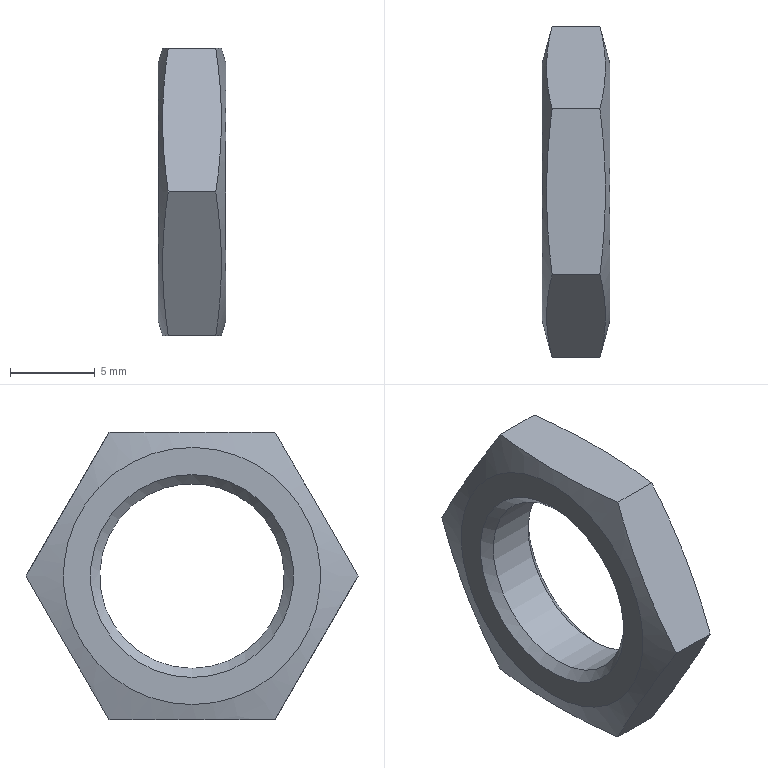Part | NX | features BREP 1 | 1 solid | 13 faces | box 4 x 19.63 x 17 mm | volume 585.312 mm3 | plane 8 | cone 4 | cylinder 1 | commonest cylinder face diameters 10.917 x1
STEP:
#1=CARTESIAN_POINT('',(4.,0.,7.6));
#2=VERTEX_POINT('',#1);
#3=CARTESIAN_POINT('',(4.,0.,0.));
#4=DIRECTION('',(-1.,0.,0.));
#5=DIRECTION('',(0.,0.,1.));
#6=AXIS2_PLACEMENT_3D('',#3,#4,#5);
#7=CIRCLE('',#6,7.6);
#8=EDGE_CURVE('',#2,#2,#7,.T.);
#9=ORIENTED_EDGE('',*,*,#8,.F.);
#10=EDGE_LOOP('',(#9));
#11=FACE_BOUND('',#10,.T.);
#12=CARTESIAN_POINT('',(4.,0.,-6.));
#13=VERTEX_POINT('',#12);
#14=CARTESIAN_POINT('',(4.,0.,0.));
#15=DIRECTION('',(1.,0.,0.));
#16=DIRECTION('',(0.,0.,-1.));
#17=AXIS2_PLACEMENT_3D('',#14,#15,#16);
#18=CIRCLE('',#17,6.);
#19=EDGE_CURVE('',#13,#13,#18,.T.);
#20=ORIENTED_EDGE('',*,*,#19,.F.);
#21=EDGE_LOOP('',(#20));
#22=FACE_BOUND('',#21,.T.);
#23=CARTESIAN_POINT('',(4.,7.6,0.));
#24=DIRECTION('',(-1.,0.,0.));
#25=DIRECTION('',(0.,0.,-1.));
#26=AXIS2_PLACEMENT_3D('',#23,#24,#25);
#27=PLANE('',#26);
#28=ADVANCED_FACE('',(#11,#22),#27,.F.);
#29=ORIENTED_EDGE('',*,*,#8,.T.);
#30=EDGE_LOOP('',(#29));
#31=FACE_BOUND('',#30,.T.);
#32=CARTESIAN_POINT('',(3.407,-9.815,0.000000038));
#33=VERTEX_POINT('',#32);
#34=CARTESIAN_POINT('',(3.407,-4.907,-8.5));
#35=VERTEX_POINT('',#34);
#36=CARTESIAN_POINT('',(3.407,-9.815,0.000000035));
#37=CARTESIAN_POINT('',(3.845,-8.179,-2.833));
#38=CARTESIAN_POINT('',(3.845,-6.543,-5.667));
#39=CARTESIAN_POINT('',(3.407,-4.907,-8.5));
#40=B_SPLINE_CURVE_WITH_KNOTS('',3,(#36,#37,#38,#39),.UNSPECIFIED.,.F.,.F.,(4,4),(0.,0.009815),.UNSPECIFIED.);
#41=EDGE_CURVE('',#33,#35,#40,.T.);
#42=ORIENTED_EDGE('',*,*,#41,.T.);
#43=CARTESIAN_POINT('',(3.407,4.907,-8.5));
#44=VERTEX_POINT('',#43);
#45=CARTESIAN_POINT('',(3.407,-4.907,-8.5));
#46=CARTESIAN_POINT('',(3.845,-1.636,-8.5));
#47=CARTESIAN_POINT('',(3.845,1.636,-8.5));
#48=CARTESIAN_POINT('',(3.407,4.907,-8.5));
#49=B_SPLINE_CURVE_WITH_KNOTS('',3,(#45,#46,#47,#48),.UNSPECIFIED.,.F.,.F.,(4,4),(0.,0.009815),.UNSPECIFIED.);
#50=EDGE_CURVE('',#35,#44,#49,.T.);
#51=ORIENTED_EDGE('',*,*,#50,.T.);
#52=CARTESIAN_POINT('',(3.407,9.815,-0.000000038));
#53=VERTEX_POINT('',#52);
#54=CARTESIAN_POINT('',(3.407,4.907,-8.5));
#55=CARTESIAN_POINT('',(3.845,6.543,-5.667));
#56=CARTESIAN_POINT('',(3.845,8.179,-2.833));
#57=CARTESIAN_POINT('',(3.407,9.815,-0.000000051));
#58=B_SPLINE_CURVE_WITH_KNOTS('',3,(#54,#55,#56,#57),.UNSPECIFIED.,.F.,.F.,(4,4),(0.,0.009815),.UNSPECIFIED.);
#59=EDGE_CURVE('',#44,#53,#58,.T.);
#60=ORIENTED_EDGE('',*,*,#59,.T.);
#61=CARTESIAN_POINT('',(3.407,4.907,8.5));
#62=VERTEX_POINT('',#61);
#63=CARTESIAN_POINT('',(3.407,9.815,-0.000000035));
#64=CARTESIAN_POINT('',(3.845,8.179,2.833));
#65=CARTESIAN_POINT('',(3.845,6.543,5.667));
#66=CARTESIAN_POINT('',(3.407,4.907,8.5));
#67=B_SPLINE_CURVE_WITH_KNOTS('',3,(#63,#64,#65,#66),.UNSPECIFIED.,.F.,.F.,(4,4),(0.,0.009815),.UNSPECIFIED.);
#68=EDGE_CURVE('',#53,#62,#67,.T.);
#69=ORIENTED_EDGE('',*,*,#68,.T.);
#70=CARTESIAN_POINT('',(3.407,-4.907,8.5));
#71=VERTEX_POINT('',#70);
#72=CARTESIAN_POINT('',(3.407,4.907,8.5));
#73=CARTESIAN_POINT('',(3.845,1.636,8.5));
#74=CARTESIAN_POINT('',(3.845,-1.636,8.5));
#75=CARTESIAN_POINT('',(3.407,-4.907,8.5));
#76=B_SPLINE_CURVE_WITH_KNOTS('',3,(#72,#73,#74,#75),.UNSPECIFIED.,.F.,.F.,(4,4),(0.,0.009815),.UNSPECIFIED.);
#77=EDGE_CURVE('',#62,#71,#76,.T.);
#78=ORIENTED_EDGE('',*,*,#77,.T.);
#79=CARTESIAN_POINT('',(3.407,-4.907,8.5));
#80=CARTESIAN_POINT('',(3.845,-6.543,5.667));
#81=CARTESIAN_POINT('',(3.845,-8.179,2.833));
#82=CARTESIAN_POINT('',(3.407,-9.815,0.000000051));
#83=B_SPLINE_CURVE_WITH_KNOTS('',3,(#79,#80,#81,#82),.UNSPECIFIED.,.F.,.F.,(4,4),(0.,0.009815),.UNSPECIFIED.);
#84=EDGE_CURVE('',#71,#33,#83,.T.);
#85=ORIENTED_EDGE('',*,*,#84,.T.);
#86=EDGE_LOOP('',(#42,#51,#60,#69,#78,#85));
#87=FACE_BOUND('',#86,.T.);
#88=CARTESIAN_POINT('',(3.403,0.,0.));
#89=DIRECTION('',(-1.,0.,0.));
#90=DIRECTION('',(0.,0.,-1.));
#91=AXIS2_PLACEMENT_3D('',#88,#89,#90);
#92=CONICAL_SURFACE('',#91,9.828,1.309);
#93=ADVANCED_FACE('',(#31,#87),#92,.T.);
#94=CARTESIAN_POINT('',(3.459,0.,-5.458));
#95=VERTEX_POINT('',#94);
#96=CARTESIAN_POINT('',(3.459,0.,0.));
#97=DIRECTION('',(1.,0.,0.));
#98=DIRECTION('',(0.,0.,-1.));
#99=AXIS2_PLACEMENT_3D('',#96,#97,#98);
#100=CIRCLE('',#99,5.458);
#101=EDGE_CURVE('',#95,#95,#100,.T.);
#102=ORIENTED_EDGE('',*,*,#101,.F.);
#103=EDGE_LOOP('',(#102));
#104=FACE_BOUND('',#103,.T.);
#105=ORIENTED_EDGE('',*,*,#19,.T.);
#106=EDGE_LOOP('',(#105));
#107=FACE_BOUND('',#106,.T.);
#108=CARTESIAN_POINT('',(4.,0.,0.));
#109=DIRECTION('',(1.,0.,0.));
#110=DIRECTION('',(0.,0.,1.));
#111=AXIS2_PLACEMENT_3D('',#108,#109,#110);
#112=CONICAL_SURFACE('',#111,6.,0.7854);
#113=ADVANCED_FACE('',(#104,#107),#112,.F.);
#114=CARTESIAN_POINT('',(0.5935,4.907,-8.5));
#115=VERTEX_POINT('',#114);
#116=CARTESIAN_POINT('',(4.,4.907,-8.5));
#117=DIRECTION('',(-1.,0.,0.));
#118=VECTOR('',#117,1000.);
#119=LINE('',#116,#118);
#120=EDGE_CURVE('',#44,#115,#119,.T.);
#121=ORIENTED_EDGE('',*,*,#120,.F.);
#122=ORIENTED_EDGE('',*,*,#50,.F.);
#123=CARTESIAN_POINT('',(0.5935,-4.907,-8.5));
#124=VERTEX_POINT('',#123);
#125=CARTESIAN_POINT('',(4.,-4.907,-8.5));
#126=DIRECTION('',(1.,0.,0.));
#127=VECTOR('',#126,1000.);
#128=LINE('',#125,#127);
#129=EDGE_CURVE('',#124,#35,#128,.T.);
#130=ORIENTED_EDGE('',*,*,#129,.F.);
#131=CARTESIAN_POINT('',(0.5935,4.907,-8.5));
#132=CARTESIAN_POINT('',(0.1552,1.636,-8.5));
#133=CARTESIAN_POINT('',(0.1552,-1.636,-8.5));
#134=CARTESIAN_POINT('',(0.5935,-4.907,-8.5));
#135=B_SPLINE_CURVE_WITH_KNOTS('',3,(#131,#132,#133,#134),.UNSPECIFIED.,.F.,.F.,(4,4),(0.,0.009815),.UNSPECIFIED.);
#136=EDGE_CURVE('',#115,#124,#135,.T.);
#137=ORIENTED_EDGE('',*,*,#136,.F.);
#138=EDGE_LOOP('',(#121,#122,#130,#137));
#139=FACE_BOUND('',#138,.T.);
#140=CARTESIAN_POINT('',(4.,-4.907,-8.5));
#141=DIRECTION('',(0.,0.,1.));
#142=DIRECTION('',(-1.,0.,0.));
#143=AXIS2_PLACEMENT_3D('',#140,#141,#142);
#144=PLANE('',#143);
#145=ADVANCED_FACE('',(#139),#144,.F.);
#146=ORIENTED_EDGE('',*,*,#41,.F.);
#147=CARTESIAN_POINT('',(0.5935,-9.815,0.));
#148=VERTEX_POINT('',#147);
#149=CARTESIAN_POINT('',(4.,-9.815,0.));
#150=DIRECTION('',(1.,0.,0.));
#151=VECTOR('',#150,1000.);
#152=LINE('',#149,#151);
#153=EDGE_CURVE('',#148,#33,#152,.T.);
#154=ORIENTED_EDGE('',*,*,#153,.F.);
#155=CARTESIAN_POINT('',(0.5935,-4.907,-8.5));
#156=CARTESIAN_POINT('',(0.1552,-6.543,-5.667));
#157=CARTESIAN_POINT('',(0.1552,-8.179,-2.833));
#158=CARTESIAN_POINT('',(0.5935,-9.815,0.));
#159=B_SPLINE_CURVE_WITH_KNOTS('',3,(#155,#156,#157,#158),.UNSPECIFIED.,.F.,.F.,(4,4),(0.,0.009815),.UNSPECIFIED.);
#160=EDGE_CURVE('',#124,#148,#159,.T.);
#161=ORIENTED_EDGE('',*,*,#160,.F.);
#162=ORIENTED_EDGE('',*,*,#129,.T.);
#163=EDGE_LOOP('',(#146,#154,#161,#162));
#164=FACE_BOUND('',#163,.T.);
#165=CARTESIAN_POINT('',(4.,-9.815,0.));
#166=DIRECTION('',(0.,0.866,0.5));
#167=DIRECTION('',(0.,0.5,-0.866));
#168=AXIS2_PLACEMENT_3D('',#165,#166,#167);
#169=PLANE('',#168);
#170=ADVANCED_FACE('',(#164),#169,.F.);
#171=ORIENTED_EDGE('',*,*,#84,.F.);
#172=CARTESIAN_POINT('',(0.5935,-4.907,8.5));
#173=VERTEX_POINT('',#172);
#174=CARTESIAN_POINT('',(4.,-4.907,8.5));
#175=DIRECTION('',(1.,0.,0.));
#176=VECTOR('',#175,1000.);
#177=LINE('',#174,#176);
#178=EDGE_CURVE('',#173,#71,#177,.T.);
#179=ORIENTED_EDGE('',*,*,#178,.F.);
#180=CARTESIAN_POINT('',(0.5935,-9.815,0.));
#181=CARTESIAN_POINT('',(0.1552,-8.179,2.833));
#182=CARTESIAN_POINT('',(0.1552,-6.543,5.667));
#183=CARTESIAN_POINT('',(0.5935,-4.907,8.5));
#184=B_SPLINE_CURVE_WITH_KNOTS('',3,(#180,#181,#182,#183),.UNSPECIFIED.,.F.,.F.,(4,4),(0.,0.009815),.UNSPECIFIED.);
#185=EDGE_CURVE('',#148,#173,#184,.T.);
#186=ORIENTED_EDGE('',*,*,#185,.F.);
#187=ORIENTED_EDGE('',*,*,#153,.T.);
#188=EDGE_LOOP('',(#171,#179,#186,#187));
#189=FACE_BOUND('',#188,.T.);
#190=CARTESIAN_POINT('',(4.,-4.907,8.5));
#191=DIRECTION('',(0.,0.866,-0.5));
#192=DIRECTION('',(0.,-0.5,-0.866));
#193=AXIS2_PLACEMENT_3D('',#190,#191,#192);
#194=PLANE('',#193);
#195=ADVANCED_FACE('',(#189),#194,.F.);
#196=ORIENTED_EDGE('',*,*,#77,.F.);
#197=CARTESIAN_POINT('',(0.5935,4.907,8.5));
#198=VERTEX_POINT('',#197);
#199=CARTESIAN_POINT('',(4.,4.907,8.5));
#200=DIRECTION('',(1.,0.,0.));
#201=VECTOR('',#200,1000.);
#202=LINE('',#199,#201);
#203=EDGE_CURVE('',#198,#62,#202,.T.);
#204=ORIENTED_EDGE('',*,*,#203,.F.);
#205=CARTESIAN_POINT('',(0.5935,-4.907,8.5));
#206=CARTESIAN_POINT('',(0.1552,-1.636,8.5));
#207=CARTESIAN_POINT('',(0.1552,1.636,8.5));
#208=CARTESIAN_POINT('',(0.5935,4.907,8.5));
#209=B_SPLINE_CURVE_WITH_KNOTS('',3,(#205,#206,#207,#208),.UNSPECIFIED.,.F.,.F.,(4,4),(0.,0.009815),.UNSPECIFIED.);
#210=EDGE_CURVE('',#173,#198,#209,.T.);
#211=ORIENTED_EDGE('',*,*,#210,.F.);
#212=ORIENTED_EDGE('',*,*,#178,.T.);
#213=EDGE_LOOP('',(#196,#204,#211,#212));
#214=FACE_BOUND('',#213,.T.);
#215=CARTESIAN_POINT('',(4.,4.907,8.5));
#216=DIRECTION('',(0.,0.,-1.));
#217=DIRECTION('',(1.,0.,0.));
#218=AXIS2_PLACEMENT_3D('',#215,#216,#217);
#219=PLANE('',#218);
#220=ADVANCED_FACE('',(#214),#219,.F.);
#221=ORIENTED_EDGE('',*,*,#68,.F.);
#222=CARTESIAN_POINT('',(0.5935,9.815,0.));
#223=VERTEX_POINT('',#222);
#224=CARTESIAN_POINT('',(4.,9.815,0.));
#225=DIRECTION('',(1.,0.,0.));
#226=VECTOR('',#225,1000.);
#227=LINE('',#224,#226);
#228=EDGE_CURVE('',#223,#53,#227,.T.);
#229=ORIENTED_EDGE('',*,*,#228,.F.);
#230=CARTESIAN_POINT('',(0.5935,4.907,8.5));
#231=CARTESIAN_POINT('',(0.1552,6.543,5.667));
#232=CARTESIAN_POINT('',(0.1552,8.179,2.833));
#233=CARTESIAN_POINT('',(0.5935,9.815,0.));
#234=B_SPLINE_CURVE_WITH_KNOTS('',3,(#230,#231,#232,#233),.UNSPECIFIED.,.F.,.F.,(4,4),(0.,0.009815),.UNSPECIFIED.);
#235=EDGE_CURVE('',#198,#223,#234,.T.);
#236=ORIENTED_EDGE('',*,*,#235,.F.);
#237=ORIENTED_EDGE('',*,*,#203,.T.);
#238=EDGE_LOOP('',(#221,#229,#236,#237));
#239=FACE_BOUND('',#238,.T.);
#240=CARTESIAN_POINT('',(4.,9.815,0.));
#241=DIRECTION('',(0.,-0.866,-0.5));
#242=DIRECTION('',(0.,-0.5,0.866));
#243=AXIS2_PLACEMENT_3D('',#240,#241,#242);
#244=PLANE('',#243);
#245=ADVANCED_FACE('',(#239),#244,.F.);
#246=ORIENTED_EDGE('',*,*,#59,.F.);
#247=ORIENTED_EDGE('',*,*,#120,.T.);
#248=CARTESIAN_POINT('',(0.5935,9.815,0.));
#249=CARTESIAN_POINT('',(0.1552,8.179,-2.833));
#250=CARTESIAN_POINT('',(0.1552,6.543,-5.667));
#251=CARTESIAN_POINT('',(0.5935,4.907,-8.5));
#252=B_SPLINE_CURVE_WITH_KNOTS('',3,(#248,#249,#250,#251),.UNSPECIFIED.,.F.,.F.,(4,4),(0.,0.009815),.UNSPECIFIED.);
#253=EDGE_CURVE('',#223,#115,#252,.T.);
#254=ORIENTED_EDGE('',*,*,#253,.F.);
#255=ORIENTED_EDGE('',*,*,#228,.T.);
#256=EDGE_LOOP('',(#246,#247,#254,#255));
#257=FACE_BOUND('',#256,.T.);
#258=CARTESIAN_POINT('',(4.,4.907,-8.5));
#259=DIRECTION('',(0.,-0.866,0.5));
#260=DIRECTION('',(0.,0.5,0.866));
#261=AXIS2_PLACEMENT_3D('',#258,#259,#260);
#262=PLANE('',#261);
#263=ADVANCED_FACE('',(#257),#262,.F.);
#264=CARTESIAN_POINT('',(0.5415,0.,-5.458));
#265=VERTEX_POINT('',#264);
#266=CARTESIAN_POINT('',(0.5415,0.,0.));
#267=DIRECTION('',(1.,0.,0.));
#268=DIRECTION('',(0.,0.,-1.));
#269=AXIS2_PLACEMENT_3D('',#266,#267,#268);
#270=CIRCLE('',#269,5.458);
#271=EDGE_CURVE('',#265,#265,#270,.T.);
#272=ORIENTED_EDGE('',*,*,#271,.F.);
#273=EDGE_LOOP('',(#272));
#274=FACE_BOUND('',#273,.T.);
#275=ORIENTED_EDGE('',*,*,#101,.T.);
#276=EDGE_LOOP('',(#275));
#277=FACE_BOUND('',#276,.T.);
#278=CARTESIAN_POINT('',(4.,0.,0.));
#279=DIRECTION('',(1.,0.,0.));
#280=DIRECTION('',(0.,0.,1.));
#281=AXIS2_PLACEMENT_3D('',#278,#279,#280);
#282=CYLINDRICAL_SURFACE('',#281,5.458);
#283=ADVANCED_FACE('',(#274,#277),#282,.F.);
#284=CARTESIAN_POINT('',(0.,0.,-7.6));
#285=VERTEX_POINT('',#284);
#286=CARTESIAN_POINT('',(0.,0.,0.));
#287=DIRECTION('',(1.,0.,0.));
#288=DIRECTION('',(0.,0.,-1.));
#289=AXIS2_PLACEMENT_3D('',#286,#287,#288);
#290=CIRCLE('',#289,7.6);
#291=EDGE_CURVE('',#285,#285,#290,.T.);
#292=ORIENTED_EDGE('',*,*,#291,.T.);
#293=EDGE_LOOP('',(#292));
#294=FACE_BOUND('',#293,.T.);
#295=ORIENTED_EDGE('',*,*,#185,.T.);
#296=ORIENTED_EDGE('',*,*,#210,.T.);
#297=ORIENTED_EDGE('',*,*,#235,.T.);
#298=ORIENTED_EDGE('',*,*,#253,.T.);
#299=ORIENTED_EDGE('',*,*,#136,.T.);
#300=ORIENTED_EDGE('',*,*,#160,.T.);
#301=EDGE_LOOP('',(#295,#296,#297,#298,#299,#300));
#302=FACE_BOUND('',#301,.T.);
#303=CARTESIAN_POINT('',(0.5971,0.,0.));
#304=DIRECTION('',(1.,0.,0.));
#305=DIRECTION('',(0.,0.,1.));
#306=AXIS2_PLACEMENT_3D('',#303,#304,#305);
#307=CONICAL_SURFACE('',#306,9.828,1.309);
#308=ADVANCED_FACE('',(#294,#302),#307,.T.);
#309=ORIENTED_EDGE('',*,*,#271,.T.);
#310=EDGE_LOOP('',(#309));
#311=FACE_BOUND('',#310,.T.);
#312=CARTESIAN_POINT('',(0.,0.,6.));
#313=VERTEX_POINT('',#312);
#314=CARTESIAN_POINT('',(0.,0.,0.));
#315=DIRECTION('',(1.,0.,0.));
#316=DIRECTION('',(0.,0.,1.));
#317=AXIS2_PLACEMENT_3D('',#314,#315,#316);
#318=CIRCLE('',#317,6.);
#319=EDGE_CURVE('',#313,#313,#318,.T.);
#320=ORIENTED_EDGE('',*,*,#319,.F.);
#321=EDGE_LOOP('',(#320));
#322=FACE_BOUND('',#321,.T.);
#323=CARTESIAN_POINT('',(0.,0.,0.));
#324=DIRECTION('',(-1.,0.,0.));
#325=DIRECTION('',(0.,0.,-1.));
#326=AXIS2_PLACEMENT_3D('',#323,#324,#325);
#327=CONICAL_SURFACE('',#326,6.,0.7854);
#328=ADVANCED_FACE('',(#311,#322),#327,.F.);
#329=ORIENTED_EDGE('',*,*,#319,.T.);
#330=EDGE_LOOP('',(#329));
#331=FACE_BOUND('',#330,.T.);
#332=ORIENTED_EDGE('',*,*,#291,.F.);
#333=EDGE_LOOP('',(#332));
#334=FACE_BOUND('',#333,.T.);
#335=CARTESIAN_POINT('',(0.,0.,0.));
#336=DIRECTION('',(1.,0.,0.));
#337=DIRECTION('',(0.,0.,1.));
#338=AXIS2_PLACEMENT_3D('',#335,#336,#337);
#339=PLANE('',#338);
#340=ADVANCED_FACE('',(#331,#334),#339,.F.);
#341=CLOSED_SHELL('',(#28,#93,#113,#145,#170,#195,#220,#245,#263,#283,#308,#328,#340));
#342=MANIFOLD_SOLID_BREP('',#341);
#343=(LENGTH_UNIT()NAMED_UNIT(*)SI_UNIT(.MILLI.,.METRE.));
#344=UNCERTAINTY_MEASURE_WITH_UNIT(LENGTH_MEASURE(0.0508),#343,'','');
#345=(NAMED_UNIT(*)PLANE_ANGLE_UNIT()SI_UNIT($,.RADIAN.));
#346=(NAMED_UNIT(*)SI_UNIT($,.STERADIAN.)SOLID_ANGLE_UNIT());
#347=(GEOMETRIC_REPRESENTATION_CONTEXT(3)GLOBAL_UNCERTAINTY_ASSIGNED_CONTEXT((#344))GLOBAL_UNIT_ASSIGNED_CONTEXT((#343,#345,#346))REPRESENTATION_CONTEXT('',''));
#348=ADVANCED_BREP_SHAPE_REPRESENTATION('',(#342),#347);